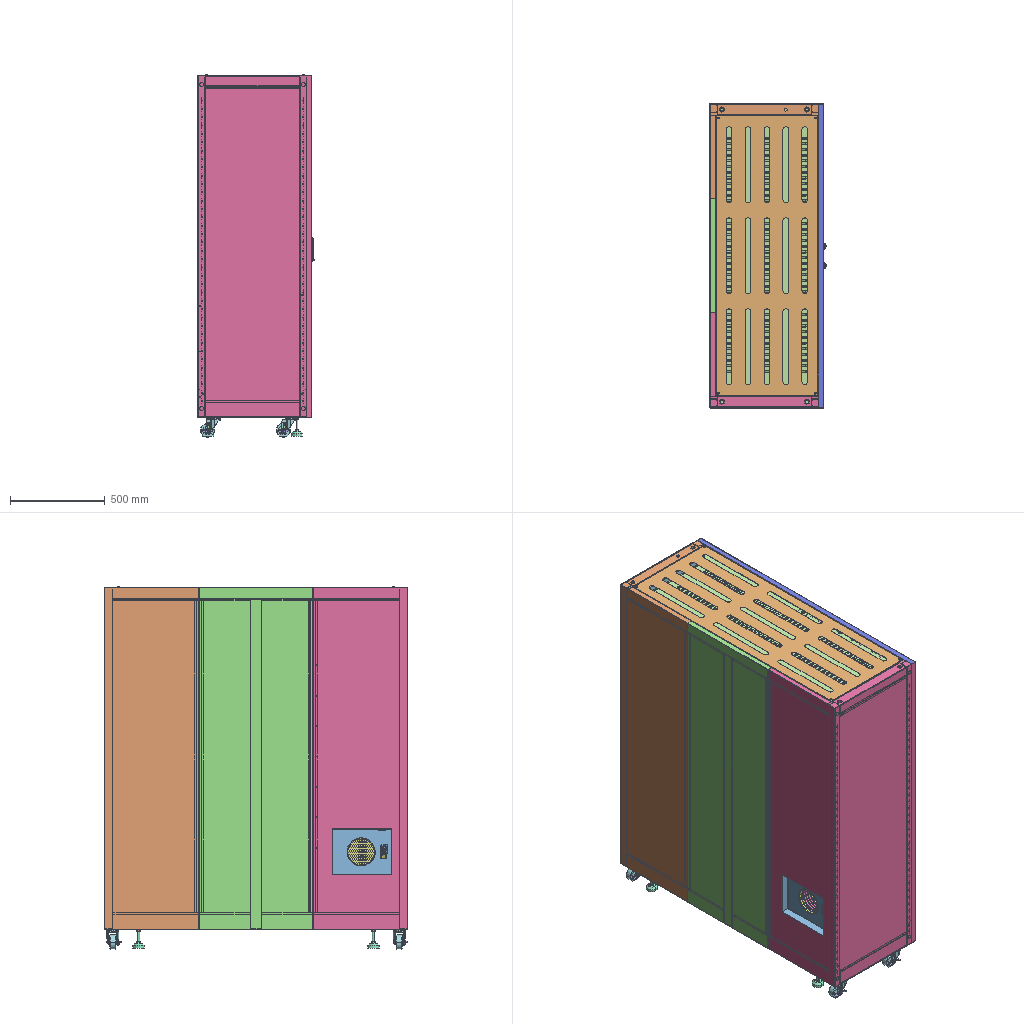Assembly | STEP file | 735 different items | 986 placed | box 612 x 1600 x 1911 mm
Parts list (item | name | quantity | parent item | size | volume), first 254 of 735 items:
1 | - | x1 | in RJWD-DY-0104_000_ASM | 10 x 10 x 37.975 mm | 923.659 mm3
2 | - | x1 | in RJWD-DY-0104_000_ASM | 10 x 10 x 37.975 mm | 923.659 mm3
3 | - | x1 | in RJWD-DY-0104_000_ASM | 10 x 10 x 37.975 mm | 923.659 mm3
4 | - | x1 | in RJWD-DY-0104_000_ASM | 2 x 2 x 1 mm | 3.142 mm3
5 | - | x1 | in RJWD-DY-0104_000_ASM | 2 x 2 x 1 mm | 3.142 mm3
6 | - | x1 | in RJWD-DY-0104_000_ASM | 537 x 1477 x 19.5 mm | 715905 mm3
7 | - | x1 | in RJWD-DY-0104_000_ASM | 10 x 10 x 37.975 mm | 923.659 mm3
8 | - | x1 | in RJWD-DY-0104_000_ASM | 2 x 2 x 1 mm | 3.142 mm3
9 | - | x1 | in RJWD-DY-0104_000_ASM | 2 x 2 x 1 mm | 3.142 mm3
10 | - | x1 | in RJWD-DY-0101_00_ASM | 498 x 92 x 78 mm | 361072 mm3
11 | - | x1 | in RJWD-DY-0101_00_ASM | 12 x 44 x 1659 mm | 107041 mm3
12 | - | x1 | in RJWD-DY-0101_00_ASM | 20 x 20 x 1.5 mm | 532.02 mm3
13 | - | x1 | in RJWD-DY-0101_00_ASM | 32 x 1480 x 131 mm | 236738 mm3
14 | - | x1 | in RJWD-DY-0101_00_ASM | 20 x 20 x 1.5 mm | 532.02 mm3
15 | - | x1 | in RJWD-DY-0101_00_ASM | 40.001 x 1598 x 110 mm | 311237 mm3
16 | - | x1 | in RJWD-DY-0101_00_ASM | 572.5 x 1598 x 16 mm | 960867 mm3
17 | RJWD-DY-0101_0002 | x5 | in RJWD-DY-0101_00_ASM | 10 x 70 x 10 mm | 871.577 mm3
18 | - | x1 | in RJWD-DY-0101_00_ASM | 24 x 27.713 x 13 mm | 3389 mm3
19 | - | x1 | in RJWD-DY-0101_00_ASM | 18 x 20.785 x 10.8 mm | 1989 mm3
20 | SOLID | x4 | in RJWD-DY-0101_300 | 37 x 45 x 1797 mm | 330738 mm3
21 | COMPOUND | x4 | in RJWD-DY-0101_300 | - | -
22 | - | x1 | in RJWD-DY-0101_00_ASM | 18 x 20.785 x 10.8 mm | 1989 mm3
23 | - | x1 | in RJWD-DY-0101_00_ASM | 104 x 1437 x 78 mm | 1081502 mm3
24 | - | x1 | in RJWD-DY-0101_00_ASM | 498 x 55 x 50 mm | 161185 mm3
25 | SOLID | x1 | - | 37 x 60 x 1739 mm | 359493 mm3
26 | COMPOUND | x1 | - | - | -
27 | - | x1 | in RJWD-DY-0101_00_ASM | 18 x 20.785 x 10.8 mm | 1989 mm3
28 | SOLID | x1 | - | 599 x 1598 x 90 mm | 1123369 mm3
29 | COMPOUND | x1 | - | - | -
30 | - | x1 | in RJWD-DY-0101_00_ASM | 600.001 x 500.001 x 1800 mm | 2227675 mm3
31 | - | x1 | in RJWD-DY-0101_00_ASM | 479 x 70 x 30 mm | 90339 mm3
32 | - | x1 | in RJWD-DY-0101_00_ASM | 40 x 600 x 1800 mm | 1173375 mm3
33 | - | x1 | in RJWD-DY-0101_00_ASM | 600.001 x 500.001 x 1800 mm | 2178717 mm3
34 | - | x1 | in RJWD-DY-0101_00_ASM | 479 x 70 x 30 mm | 90339 mm3
35 | - | x1 | in RJWD-DY-0101_00_ASM | 18 x 20.785 x 10.8 mm | 1989 mm3
36 | - | x1 | in RJWD-DY-0101_00_ASM | 498 x 80.2 x 78 mm | 347718 mm3
37 | - | x1 | in RJWD-DY-0101_00_ASM | 12 x 44 x 1659 mm | 107041 mm3
38 | - | x1 | in RJWD-DY-0101_00_ASM | 24 x 27.713 x 13 mm | 3389 mm3
39 | - | x1 | in RJWD-DY-0101_00_ASM | 498 x 55 x 50 mm | 160582 mm3
40 | - | x1 | in RJWD-DY-0101_00_ASM | 24 x 27.713 x 13 mm | 3389 mm3
41 | - | x1 | in RJWD-DY-0101_00_ASM | 37 x 60 x 1739 mm | 359909 mm3
42 | - | x1 | in RJWD-DY-0101_00_ASM | 20 x 20 x 1.5 mm | 532.02 mm3
43 | - | x1 | in RJWD-DY-0101_00_ASM | 20 x 20 x 1.5 mm | 532.02 mm3
44 | - | x1 | in RJWD-DY-0101_00_ASM | 24 x 27.713 x 13 mm | 3389 mm3
45 | - | x1 | in RJWD-DY-0101_00_ASM | 104 x 1437 x 78 mm | 1081502 mm3
46 | RJWD-DY-0101_0003 | x3 | in RJWD-DY-0101_00_ASM | 220 x 15 x 20 mm | 3858 mm3
47 | RJWD-DY-01010001 | x1 | in RJWD-DY-0101_00_ASM | 312.4 x 242.4 x 75 mm | 132718 mm3
48 | - | x1 | in RJWD-DY-0101_00_ASM | 10 x 60 x 10 mm | 771.555 mm3
49 | _GFEEA-D60-M12-L125-DUMMY | x4 | in GFEEA-D60-M12-L125_1_ASM | - | -
50 | _GFEEA-D60-M12-L125-1 | x4 | in GFEEA-D60-M12-L125_1_ASM | 60 x 157 x 60 mm | 76084 mm3
51 | _GFEEA-D60-M12-L125-2 | x4 | in GFEEA-D60-M12-L125_1_ASM | 19 x 10 x 21.939 mm | 2279 mm3
52 | JDC-75-3 | x4 | in JDC-75_ASM | 74.72 x 27.5 x 19.44 mm | 3290 mm3
53 | JDC-75-2 | x4 | in JDC-75_ASM | 25.398 x 59.274 x 36 mm | 3330 mm3
54 | JDC-75-5 | x4 | in JDC-75_ASM | 11.547 x 10 x 3.2 mm | 211.321 mm3
55 | JDC-75-1 | x4 | in JDC-75_ASM | 122 x 106 x 67 mm | 215545 mm3
56 | JDC-75-4 | x4 | in JDC-75_ASM | 6 x 7 x 6 mm | 146.084 mm3
57 | 0001 | x1 | in RJWD-DY-0101_00_ASM | 10 x 10 x 520 mm | 9724 mm3
58 | SOLID | x1 | in 0002 | 48 x 270 x 317 mm | 394936 mm3
59 | COMPOUND | x1 | in 0002 | - | -
60 | RJWD-DY-0101_30002 | x2 | in RJWD-DY-0101_00_ASM | 150 x 10 x 20 mm | 1872 mm3
61 | RJWD-DY-0101_20001 | x2 | in RJWD-DY-0101_00_ASM, RJWD-DY-0115-0001_ASM | 120 x 10 x 20 mm | 1571 mm3
62 | SOLID | x4 | in M1000 | 18.475 x 16 x 9.5 mm | 1567 mm3
63 | SHELL | x4 | in M1000 | - | -
64 | 000 | x1 | in RJWD-DY-0101_00_ASM | 300 x 220 x 20 mm | 1310952 mm3
65 | RJWD-DY-0111_00 | x3 | in RJWD-DY-01_0001_ASM | 24 x 537.5 x 71.5 mm | 60134 mm3
66 | SOLID | x1 | in RJWD-DY-0108_000 | 493 x 75 x 702 mm | 761842 mm3
67 | COMPOUND | x1 | in RJWD-DY-0108_000 | - | -
68 | RJWD-DY-0108_0003 | x4 | in RJWD-DY-0108_000_ASM | 38 x 1 x 20 mm | 730.064 mm3
69 | _2000 | x2 | in RJWD-DY-0108_000_ASM | 426.4 x 3 x 60.8 mm | 11438 mm3
70 | _3000 | x1 | in RJWD-DY-0108_000_ASM | 426.4 x 3 x 60.8 mm | 12335 mm3
71 | _0-1000 | x1 | in RJWD-DY-0108_000_ASM | 278 x 12 x 188 mm | 42731 mm3
72 | M40001 | x12 | in RJWD-DY-0108_000_ASM | 7.9 x 7.9 x 2.97 mm | 98.242 mm3
73 | RJWD-DY-0105--0001 | x1 | in RJWD-DY-0105_-0001_ASM | 728.7 x 458 x 509.2 mm | 1538586 mm3
74 | RJWD-DY-010607_3D0001 | x28 | in RJWD-DY-0105_-0001_ASM, RJWD-DY-0106_-0001_ASM, RJWD-DY-0107_-0001_ASM | 78.111 x 40 x 80.345 mm | 35899 mm3
75 | RJWD-DY-0109_-0001 | x1 | in RJWD-DY-0109_0001_ASM | 722 x 555.2 x 25 mm | 417115 mm3
76 | RJWD-DY-0112_X2_4F20611F56685_1 | x1 | in RJWD-DY-0112_0001_ASM | 1 x 166 x 30 mm | 4869 mm3
77 | RJWD-DY-0112_X2_4F20611F56685_2 | x1 | in RJWD-DY-0112_0001_ASM | 10.8 x 137.602 x 10 mm | 1934 mm3
78 | RJWD-DY-0114_X2_75356C145B89_10 | x1 | in RJWD-DY-0114_0001_ASM | 113.5 x 434 x 340 mm | 170020 mm3
79 | RJWD-DY-0114_X2_75356C145B898_5 | x2 | in RJWD-DY-0114_0001_ASM | 48.998 x 1 x 99.996 mm | 2450 mm3
80 | RJWD-DY-0114_X2_75356C145B898_7 | x1 | in RJWD-DY-0114_0001_ASM | 10 x 10 x 290 mm | 5331 mm3
81 | RJWD-DY-0106--0001 | x1 | in RJWD-DY-0106_-0001_ASM | 728.7 x 458 x 509.2 mm | 1538585 mm3
82 | RJWD-DY-0107--0001 | x1 | in RJWD-DY-0107_-0001_ASM | 728.7 x 458 x 349.2 mm | 1552661 mm3
83 | - | x1 | - | 4 x 509 x 1099 mm | 2237564 mm3
84 | - | x1 | - | 4 x 509.4 x 200.9 mm | 409354 mm3
85 | _X2_751F4E45_X0_LG003_X2_8-1054 | x1 | in _X2_5DE667DC95E88FDE67469501_X0_ASM | 8.003 x 14 x 760 mm | 36967 mm3
86 | _X2_751F4E45_X0_MS731-1_X2_8F_1 | x2 | in _X2_751F4E45_X0_MS731-1_X2_8FDE_ASM | 14.5 x 17.374 x 15.879 mm | 1874 mm3
87 | _X2_751F4E45_X0_MS731-1_X2_8F_3 | x2 | in _X2_751F4E45_X0_MS731-1_X2_8FDE_ASM | 15.1 x 4.709 x 15.173 mm | 73.288 mm3
88 | _X2_751F4E45_X0_MS731-1_X2_8F_4 | x2 | in _X2_751F4E45_X0_MS731-1_X2_8FDE_ASM | 17.2 x 2.5 x 17.2 mm | 530.64 mm3
89 | _X2_751F4E45_X0_MS731-1_X2_8F_5 | x2 | in _X2_751F4E45_X0_MS731-1_X2_8FDE_ASM | 25.8 x 35.5 x 24.1 mm | 3742 mm3
90 | _X2_751F4E45_X0_MS731-1_X2_8F_6 | x2 | in _X2_751F4E45_X0_MS731-1_X2_8FDE_ASM | 30 x 1 x 128 mm | 892.292 mm3
91 | _X2_751F4E45_X0_MS731-1_X2_8F_7 | x2 | in _X2_751F4E45_X0_MS731-1_X2_8FDE_ASM | 44 x 3 x 18 mm | 1686 mm3
92 | _X2_751F4E45_X0_MS731-1_X2_8F_8 | x2 | in _X2_751F4E45_X0_MS731-1_X2_8FDE_ASM | 17.395 x 18 x 83 mm | 8684 mm3
93 | _X2_751F4E45_X0_MS731-1_X2_8F_9 | x2 | in _X2_751F4E45_X0_MS731-1_X2_8FDE_ASM | 29 x 6 x 35 mm | 2353 mm3
94 | _X2_751F4E45_X0_MS731-1_X2_8_10 | x2 | in _X2_751F4E45_X0_MS731-1_X2_8FDE_ASM | 8.5 x 19.466 x 8.5 mm | 271.985 mm3
95 | _X2_751F4E45_X0_MS731-1_X2_8_11 | x2 | in _X2_751F4E45_X0_MS731-1_X2_8FDE_ASM | 22.3 x 4.5 x 4.5 mm | 158.929 mm3
96 | _X2_751F4E45_X0_MS731-1_X2_8_12 | x2 | in _X2_751F4E45_X0_MS731-1_X2_8FDE_ASM | 12 x 12.2 x 12 mm | 416.607 mm3
97 | _X2_751F4E45_X0_MS731-1_X2_8_13 | x2 | in _X2_751F4E45_X0_MS731-1_X2_8FDE_ASM | 31 x 25.045 x 130 mm | 21766 mm3
98 | _X2_751F4E45_X0_MS731-1_X2_8_14 | x2 | in _X2_751F4E45_X0_MS731-1_X2_8FDE_ASM | 8.5 x 19.466 x 8.5 mm | 271.985 mm3
99 | _X2_751F4E45_X0_MS731-1_X2_8_15 | x2 | in _X2_751F4E45_X0_MS731-1_X2_8FDE_ASM | 27 x 14.4 x 37.3 mm | 4925 mm3
100 | _X2_751F4E45_X0_MS731-1_X2_8_16 | x2 | in _X2_751F4E45_X0_MS731-1_X2_8FDE_ASM | 12 x 12.2 x 12 mm | 416.607 mm3
101 | _X2_751F4E45_X0_MS731-1_X2_8_17 | x2 | in _X2_751F4E45_X0_MS731-1_X2_8FDE_ASM | 7 x 2.3 x 7 mm | 15.077 mm3
102 | _X2_751F4E45_X0_MS731-1_X2_8_18 | x2 | in _X2_751F4E45_X0_MS731-1_X2_8FDE_ASM | 12 x 12.2 x 12 mm | 416.607 mm3
103 | _X2_751F4E45_X0_MS731-1_X2_8_19 | x2 | in _X2_751F4E45_X0_MS731-1_X2_8FDE_ASM | 7 x 2.3 x 7 mm | 15.077 mm3
104 | _X2_751F4E45_X0_MS731-1_X2_8_20 | x2 | in _X2_751F4E45_X0_MS731-1_X2_8FDE_ASM | 17 x 13.5 x 26 mm | 1619 mm3
105 | _X2_751F4E45_X0_MS731-1_X2_8_21 | x2 | in _X2_751F4E45_X0_MS731-1_X2_8FDE_ASM | 10 x 1 x 10 mm | 58.905 mm3
106 | _X2_751F4E45_X0_MS731-1_X2_8_22 | x2 | in _X2_751F4E45_X0_MS731-1_X2_8FDE_ASM | 27 x 11.4 x 37.3 mm | 4808 mm3
107 | _X2_751F4E45_X0_MS731-1_X2_8_23 | x2 | in _X2_751F4E45_X0_MS731-1_X2_8FDE_ASM | 16.8 x 3 x 3 mm | 118.356 mm3
108 | _X2_751F4E45_X0_MS731-1_X2_8_24 | x2 | in _X2_751F4E45_X0_MS731-1_X2_8FDE_ASM | 10 x 1 x 10 mm | 58.905 mm3
109 | _X2_751F4E45_X0_MS731-1_X2_8_25 | x2 | in _X2_751F4E45_X0_MS731-1_X2_8FDE_ASM | 22.757 x 2.5 x 22.757 mm | 558.462 mm3
110 | _X2_751F4E45_X0_MS731-1_X2_8_26 | x2 | in _X2_751F4E45_X0_MS731-1_X2_8FDE_ASM | 5.5 x 5 x 5.5 mm | 41.588 mm3
111 | _X2_751F4E45_X0_MS731-1_X2_8_27 | x2 | in _X2_751F4E45_X0_MS731-1_X2_8FDE_ASM | 17.4 x 26.019 x 28.81 mm | 2994 mm3
112 | _X2_751F4E45_X0_MS731-1_X2_8_29 | x2 | in _X2_751F4E45_X0_MS731-1_X2_8FDE_ASM | 5.5 x 5 x 5.5 mm | 41.588 mm3
113 | _X2_751F4E45_X0_RG004-3_X2_5BFC | x4 | in _X2_5DE667DC95E88FDE67469501_X0_ASM, _X2_53F367DC95E88FDE67469501_X0_ASM | 30 x 20 x 36 mm | 14717 mm3
114 | _X2_751F4E45_X0_LG003_X2_8-1051 | x1 | in _X2_5DE667DC95E88FDE67469501_X0_ASM | 14 x 8.003 x 719 mm | 34906 mm3
115 | - | x1 | in RJWD-DY-0102_000_ASM | 18.5 x 511.5 x 98.4 mm | 54675 mm3
116 | - | x1 | in RJWD-DY-0102_000_ASM | 15 x 4 x 4 mm | 187.056 mm3
117 | - | x1 | in RJWD-DY-0102_000_ASM | 18.5 x 511.5 x 34.7 mm | 20752 mm3
118 | - | x1 | in RJWD-DY-0102_000_ASM | 10 x 527.858 x 25 mm | 17063 mm3
119 | RJWD-DY-0102_X2_5DE667DC95E8_11 | x1 | in RJWD-DY-0102_000_ASM | 15 x 4 x 4 mm | 187.056 mm3
120 | RJWD-DY-0102_X2_5DE667DC95E8_12 | x1 | in RJWD-DY-0102_000_ASM | 10 x 501.004 x 192.504 mm | 49501 mm3
121 | RJWD-DY-0102_X2_5DE667DC95E8_14 | x1 | in RJWD-DY-0102_000_ASM | 11.681 x 8 x 8 mm | 225.554 mm3
122 | RJWD-DY-0102_X2_5DE667DC95E8_17 | x1 | in RJWD-DY-0102_000_ASM | 21 x 756.2 x 1704 mm | 844463 mm3
123 | RJWD-DY-0102_X2_5DE667DC95E8_20 | x1 | in RJWD-DY-0102_000_ASM | 15 x 4 x 4 mm | 187.056 mm3
124 | RJWD-DY-0102_X2_5DE667DC95E8_21 | x1 | in RJWD-DY-0102_000_ASM | 11.681 x 8 x 8 mm | 225.554 mm3
125 | RJWD-DY-0102_X2_5DE667DC95E8_22 | x1 | in RJWD-DY-0102_000_ASM | 10 x 501.011 x 1091 mm | 114606 mm3
126 | RJWD-DY-0102_X2_5DE667DC95E8_24 | x1 | in RJWD-DY-0102_000_ASM | 10 x 10 x 18 mm | 607.492 mm3
127 | RJWD-DY-0102_X2_5DE667DC95E8_25 | x1 | in RJWD-DY-0102_000_ASM | 22 x 6 x 6 mm | 613.658 mm3
128 | RJWD-DY-0102_X2_5DE667DC95E8_26 | x1 | in RJWD-DY-0102_000_ASM | 10 x 25 x 219.358 mm | 6666 mm3
129 | RJWD-DY-0102_X2_5DE667DC95E8_27 | x1 | in RJWD-DY-0102_000_ASM | 11.681 x 8 x 8 mm | 225.554 mm3
130 | RJWD-DY-0102_X2_5DE667DC95E8_28 | x1 | in RJWD-DY-0102_000_ASM | 10 x 25 x 1118 mm | 36787 mm3
131 | RJWD-DY-0102_X2_5DE667DC95E8_30 | x1 | in RJWD-DY-0102_000_ASM | 10 x 24 x 62.5 mm | 2502 mm3
132 | RJWD-DY-0102_X2_5DE667DC95E8_33 | x1 | in RJWD-DY-0102_000_ASM | 11.681 x 8 x 8 mm | 225.554 mm3
133 | RJWD-DY-0102_X2_5DE667DC95E8_34 | x1 | in RJWD-DY-0102_000_ASM | 10 x 25 x 1118 mm | 36787 mm3
134 | RJWD-DY-0102_X2_5DE667DC95E8_35 | x1 | in RJWD-DY-0102_000_ASM | 18.5 x 511.5 x 34.7 mm | 20752 mm3
135 | RJWD-DY-0102_X2_5DE667DC95E8_37 | x1 | in RJWD-DY-0102_000_ASM | 5.7 x 17.85 x 93.35 mm | 2651 mm3
136 | RJWD-DY-0102_X2_5DE667DC95E8_38 | x1 | in RJWD-DY-0102_000_ASM | 22 x 6 x 6 mm | 613.658 mm3
137 | RJWD-DY-0102_X2_5DE667DC95E8_39 | x1 | in RJWD-DY-0102_000_ASM | 10 x 545 x 243 mm | 139493 mm3
138 | RJWD-DY-0102_X2_5DE667DC95E8_41 | x1 | in RJWD-DY-0102_000_ASM | 11.681 x 8 x 8 mm | 225.554 mm3
139 | RJWD-DY-0102_X2_5DE667DC95E8_42 | x1 | in RJWD-DY-0102_000_ASM | 10 x 527.858 x 25 mm | 17063 mm3
140 | RJWD-DY-0102_X2_5DE667DC95E8_44 | x1 | in RJWD-DY-0102_000_ASM | 3 x 752 x 1702 mm | 218115 mm3
141 | RJWD-DY-0102_X2_5DE667DC95E8_45 | x1 | in RJWD-DY-0102_000_ASM | 22 x 6 x 6 mm | 613.658 mm3
142 | RJWD-DY-0102_M4X800 | x28 | in RJWD-DY-0102_000_ASM | 11.681 x 8 x 8 mm | 225.554 mm3
143 | RJWD-DY-0102_X2_5DE667DC95E8_48 | x1 | in RJWD-DY-0102_000_ASM | 11.681 x 8 x 8 mm | 225.554 mm3
144 | RJWD-DY-0102_X2_5DE667DC95E8_49 | x1 | in RJWD-DY-0102_000_ASM | 18.5 x 134.2 x 1677 mm | 204085 mm3
145 | RJWD-DY-0102_X2_5DE667DC95E8_50 | x1 | in RJWD-DY-0102_000_ASM | 22 x 6 x 6 mm | 613.658 mm3
146 | RJWD-DY-0102_X2_5DE667DC95E8_53 | x1 | in RJWD-DY-0102_000_ASM | 10 x 25 x 219.358 mm | 6666 mm3
147 | RJWD-DY-0102_X2_5DE667DC95E8_55 | x1 | in RJWD-DY-0102_000_ASM | 11.681 x 8 x 8 mm | 225.554 mm3
148 | RJWD-DY-0102_X2_5DE667DC95E8_56 | x1 | in RJWD-DY-0102_000_ASM | 30.5 x 133.9 x 1677 mm | 217200 mm3
149 | RJWD-DY-0102_X2_5DE667DC95E8_60 | x1 | in RJWD-DY-0102_000_ASM | 11.681 x 8 x 8 mm | 225.554 mm3
150 | RJWD-DY-0102_X2_5DE667DC95E8_61 | x1 | in RJWD-DY-0102_000_ASM | 18.5 x 511.5 x 98.4 mm | 54675 mm3
151 | RJWD-DY-0102_X2_5DE667DC95E8_64 | x1 | in RJWD-DY-0102_000_ASM | 15 x 4 x 4 mm | 187.056 mm3
152 | - | x1 | - | 4 x 509 x 1099 mm | 2237564 mm3
153 | - | x1 | - | 4 x 509.2 x 201.1 mm | 409600 mm3
154 | - | x1 | in RJWD-DY-0103_000_ASM | 11.681 x 8 x 8 mm | 225.551 mm3
155 | - | x1 | in RJWD-DY-0103_000_ASM | 11.681 x 8 x 8 mm | 225.551 mm3
156 | - | x1 | in RJWD-DY-0103_000_ASM | 11.681 x 8 x 8 mm | 225.554 mm3
157 | - | x1 | in RJWD-DY-0103_000_ASM | 11.681 x 8 x 8 mm | 225.551 mm3
158 | - | x1 | in RJWD-DY-0103_000_ASM | 11.681 x 8 x 8 mm | 225.551 mm3
159 | - | x1 | in RJWD-DY-0103_000_ASM | 3 x 754 x 1702 mm | 218295 mm3
160 | - | x1 | in RJWD-DY-0103_000_ASM | 11.681 x 8 x 8 mm | 225.551 mm3
161 | - | x1 | in RJWD-DY-0103_000_ASM | 11.681 x 8 x 8 mm | 225.551 mm3
162 | - | x1 | in RJWD-DY-0103_000_ASM | 11.681 x 8 x 8 mm | 225.551 mm3
163 | RJWD-DY-0103_X2_53F367DC95E8_10 | x1 | in RJWD-DY-0103_000_ASM | 5.7 x 20.85 x 93.35 mm | 2686 mm3
164 | RJWD-DY-0103_X2_53F367DC95E8_11 | x1 | in RJWD-DY-0103_000_ASM | 11.681 x 8 x 8 mm | 225.551 mm3
165 | RJWD-DY-0103_X2_53F367DC95E8_12 | x1 | in RJWD-DY-0103_000_ASM | 10 x 501.011 x 1091 mm | 114606 mm3
166 | RJWD-DY-0103_X2_53F367DC95E8_13 | x1 | in RJWD-DY-0103_000_ASM | 11.681 x 8 x 8 mm | 225.551 mm3
167 | RJWD-DY-0103_X2_53F367DC95E8_14 | x1 | in RJWD-DY-0103_000_ASM | 11.681 x 8 x 8 mm | 225.551 mm3
168 | RJWD-DY-0103_X2_53F367DC95E8_15 | x1 | in RJWD-DY-0103_000_ASM | 11.681 x 8 x 8 mm | 225.551 mm3
169 | RJWD-DY-0103_X2_53F367DC95E8_16 | x1 | in RJWD-DY-0103_000_ASM | 11.681 x 8 x 8 mm | 225.551 mm3
170 | RJWD-DY-0103_X2_53F367DC95E8_17 | x1 | in RJWD-DY-0103_000_ASM | 10 x 527.858 x 25 mm | 17063 mm3
171 | RJWD-DY-0103_X2_53F367DC95E8_18 | x1 | in RJWD-DY-0103_000_ASM | 11.681 x 8 x 8 mm | 225.551 mm3
172 | RJWD-DY-0103_X2_53F367DC95E8_19 | x1 | in RJWD-DY-0103_000_ASM | 11.681 x 8 x 8 mm | 225.551 mm3
173 | RJWD-DY-0103_X2_53F367DC95E8_20 | x1 | in RJWD-DY-0103_000_ASM | 11.681 x 8 x 8 mm | 225.551 mm3
174 | RJWD-DY-0103_X2_53F367DC95E8_21 | x1 | in RJWD-DY-0103_000_ASM | 11.681 x 8 x 8 mm | 225.551 mm3
175 | RJWD-DY-0103_X2_53F367DC95E8_22 | x1 | in RJWD-DY-0103_000_ASM | 11.681 x 8 x 8 mm | 225.551 mm3
176 | RJWD-DY-0103_X2_53F367DC95E8_23 | x1 | in RJWD-DY-0103_000_ASM | 10 x 545 x 243 mm | 139572 mm3
177 | RJWD-DY-0103_X2_53F367DC95E8_24 | x1 | in RJWD-DY-0103_000_ASM | 10 x 24 x 62.5 mm | 2502 mm3
178 | RJWD-DY-0103_X2_53F367DC95E8_25 | x1 | in RJWD-DY-0103_000_ASM | 10 x 10 x 18 mm | 607.492 mm3
179 | RJWD-DY-0103_X2_53F367DC95E8_26 | x1 | in RJWD-DY-0103_000_ASM | 10 x 25 x 1118 mm | 36806 mm3
180 | RJWD-DY-0103_X2_53F367DC95E8_27 | x1 | in RJWD-DY-0103_000_ASM | 10 x 25 x 219.358 mm | 6666 mm3
181 | RJWD-DY-0103_X2_53F367DC95E8_28 | x1 | in RJWD-DY-0103_000_ASM | 11.681 x 8 x 8 mm | 225.551 mm3
182 | RJWD-DY-0103_X2_53F367DC95E8_29 | x1 | in RJWD-DY-0103_000_ASM | 18.5 x 511.5 x 34.7 mm | 20752 mm3
183 | RJWD-DY-0103_X2_53F367DC95E8_30 | x1 | in RJWD-DY-0103_000_ASM | 11.681 x 8 x 8 mm | 225.551 mm3
184 | RJWD-DY-0103_X2_53F367DC95E8_31 | x1 | in RJWD-DY-0103_000_ASM | 11.681 x 8 x 8 mm | 225.554 mm3
185 | RJWD-DY-0103_X2_53F367DC95E8_32 | x1 | in RJWD-DY-0103_000_ASM | 11.681 x 8 x 8 mm | 225.551 mm3
186 | RJWD-DY-0103_X2_53F367DC95E8_33 | x1 | in RJWD-DY-0103_000_ASM | 11.681 x 8 x 8 mm | 225.551 mm3
187 | RJWD-DY-0103_X2_53F367DC95E8_34 | x1 | in RJWD-DY-0103_000_ASM | 30.5 x 133.9 x 1677 mm | 217200 mm3
188 | RJWD-DY-0103_X2_53F367DC95E8_35 | x1 | in RJWD-DY-0103_000_ASM | 11.681 x 8 x 8 mm | 225.551 mm3
189 | RJWD-DY-0103_X2_53F367DC95E8_36 | x1 | in RJWD-DY-0103_000_ASM | 11.681 x 8 x 8 mm | 225.551 mm3
190 | RJWD-DY-0103_X2_53F367DC95E8_37 | x1 | in RJWD-DY-0103_000_ASM | 11.681 x 8 x 8 mm | 225.551 mm3
191 | RJWD-DY-0103_X2_53F367DC95E8_38 | x1 | in RJWD-DY-0103_000_ASM | 11.681 x 8 x 8 mm | 225.551 mm3
192 | RJWD-DY-0103_X2_53F367DC95E8_39 | x1 | in RJWD-DY-0103_000_ASM | 18.5 x 134.2 x 1677 mm | 204085 mm3
193 | RJWD-DY-0103_X2_53F367DC95E8_40 | x1 | in RJWD-DY-0103_000_ASM | 10 x 25 x 1118 mm | 36806 mm3
194 | RJWD-DY-0103_X2_53F367DC95E8_41 | x1 | in RJWD-DY-0103_000_ASM | 11.681 x 8 x 8 mm | 225.554 mm3
195 | RJWD-DY-0103_X2_53F367DC95E8_42 | x1 | in RJWD-DY-0103_000_ASM | 10 x 527.858 x 25 mm | 17063 mm3
196 | RJWD-DY-0103_X2_53F367DC95E8_43 | x1 | in RJWD-DY-0103_000_ASM | 11.681 x 8 x 8 mm | 225.554 mm3
197 | RJWD-DY-0103_X2_53F367DC95E8_44 | x1 | in RJWD-DY-0103_000_ASM | 11.681 x 8 x 8 mm | 225.551 mm3
198 | RJWD-DY-0103_X2_53F367DC95E8_45 | x1 | in RJWD-DY-0103_000_ASM | 18.5 x 511.5 x 34.7 mm | 20752 mm3
199 | RJWD-DY-0103_X2_53F367DC95E8_46 | x1 | in RJWD-DY-0103_000_ASM | 11.681 x 8 x 8 mm | 225.551 mm3
200 | RJWD-DY-0103_X2_53F367DC95E8_47 | x1 | in RJWD-DY-0103_000_ASM | 10 x 25 x 219.358 mm | 6666 mm3
201 | RJWD-DY-0103_X2_53F367DC95E8_48 | x1 | in RJWD-DY-0103_000_ASM | 26.5 x 775.2 x 1704 mm | 873122 mm3
202 | RJWD-DY-0103_X2_53F367DC95E8_49 | x1 | in RJWD-DY-0103_000_ASM | 10 x 501.004 x 192.504 mm | 49501 mm3
203 | RJWD-DY-0103_X2_53F367DC95E8_50 | x1 | in RJWD-DY-0103_000_ASM | 11.681 x 8 x 8 mm | 225.551 mm3
204 | RJWD-DY-0103_X2_53F367DC95E8_51 | x1 | in RJWD-DY-0103_000_ASM | 18.5 x 511.5 x 98.4 mm | 54675 mm3
205 | RJWD-DY-0103_X2_53F367DC95E8_52 | x1 | in RJWD-DY-0103_000_ASM | 11.681 x 8 x 8 mm | 225.551 mm3
206 | RJWD-DY-0103_X2_53F367DC95E8_53 | x1 | in RJWD-DY-0103_000_ASM | 11.681 x 8 x 8 mm | 225.551 mm3
207 | RJWD-DY-0103_X2_53F367DC95E8_54 | x1 | in RJWD-DY-0103_000_ASM | 11.681 x 8 x 8 mm | 225.551 mm3
208 | RJWD-DY-0103_X2_53F367DC95E8_55 | x1 | in RJWD-DY-0103_000_ASM | 11.681 x 8 x 8 mm | 225.551 mm3
209 | RJWD-DY-0103_X2_53F367DC95E8_56 | x1 | in RJWD-DY-0103_000_ASM | 18.5 x 511.5 x 98.4 mm | 54675 mm3
210 | RJWD-DY-0115-0002 | x1 | in RJWD-DY-0115-0001_ASM | 291 x 201 x 191.2 mm | 195011 mm3
211 | RJWD-DY-0113--0001 | x1 | in RJWD-DY-01_0001_ASM | 152 x 132 x 1 mm | 18679 mm3
212 | RJWD-DY-0110_0002 | x1 | in RJWD-DY-0110_0001_ASM | 720 x 548 x 32 mm | 426784 mm3
213 | CHAXIAO6-2_86_1 | x1 | in CHAXIAO6-2_86_ASM | 62.5 x 24 x 10 mm | 2502 mm3
214 | CHAXIAO6-2_86_2 | x1 | in CHAXIAO6-2_86_ASM | 93.35 x 17.85 x 5.7 mm | 2651 mm3
215 | CHAXIAO6-1_78_1 | x1 | in CHAXIAO6-1_78_ASM | 62.5 x 24 x 10 mm | 2502 mm3
216 | CHAXIAO6-1_78_2 | x1 | in CHAXIAO6-1_78_ASM | 93.35 x 20.85 x 5.7 mm | 2686 mm3
217 | SOLID | x9 | in ISO7045-M4X12-4_8 | 15.088 x 8 x 8 mm | 268.486 mm3
218 | SHELL | x9 | in ISO7045-M4X12-4_8 | - | -
219 | DINENISO7092-4 | x13 | in RJWD-DY-01_0001_ASM, 00-RJWD-DY_-10280001_ASM | 0.55 x 8 x 8 mm | 19.659 mm3
220 | DMG10600T070_01WTC_X2_8FEA658_1 | x1 | in DMG10600T070_01WTC_X2_8FEA65875_ASM | 99.7 x 164.6 x 1.775 mm | 25129 mm3
221 | DMG10600T070_01WTC_X2_8FEA658_2 | x1 | in DMG10600T070_01WTC_X2_8FEA65875_ASM | 105.41 x 190.5 x 13.675 mm | 120263 mm3
222 | DMG10600T070_01WTC_X2_8FEA658_3 | x1 | in DMG10600T070_01WTC_X2_8FEA65875_ASM | 105.41 x 190.5 x 7.4 mm | 40629 mm3
223 | DMG10600T070_01WTC_X2_8FEA658_4 | x1 | in DMG10600T070_01WTC_X2_8FEA65875_ASM | 101.5 x 166.2 x 8.5 mm | 2112 mm3
224 | DMG10600T070_01WTC_X2_8FEA658_5 | x1 | in DMG10600T070_01WTC_X2_8FEA65875_ASM | 99.96 x 164.86 x 3.3 mm | 52395 mm3
225 | RJ-HMS7-01_X2_58F34F5394A391D_2 | x1 | in RJ-HMS7-01_X2_58F34F5394A391D17_ASM | 2 x 200 x 140 mm | 19939 mm3
226 | RJ-HMS7-01_X2_58F34F5394A391D_4 | x1 | in RJ-HMS7-01_X2_58F34F5394A391D17_ASM | 1 x 180 x 110 mm | 6715 mm3
227 | RJ-HMS7-01_X2_58F34F5394A391D_1 | x1 | in RJ-HMS7-01_X2_58F34F5394A391D17_ASM | 5.5 x 5.39 x 5.39 mm | 86.619 mm3
228 | RJ-HMS7-01_X2_58F34F5394A391D_3 | x1 | in RJ-HMS7-01_X2_58F34F5394A391D17_ASM | 5.5 x 5.39 x 5.39 mm | 86.619 mm3
229 | RJ-HMS7-01_X2_58F34F5394A391D_5 | x1 | in RJ-HMS7-01_X2_58F34F5394A391D17_ASM | 5.5 x 5.39 x 5.39 mm | 86.619 mm3
230 | RJ-HMS7-01_X2_58F34F5394A391D_6 | x1 | in RJ-HMS7-01_X2_58F34F5394A391D17_ASM | 5.5 x 5.39 x 5.39 mm | 86.619 mm3
231 | ASSEMBLY_GB_T_9074_4_M3X8_2 | x4 | - | 0.8 x 5.4 x 5.4 mm | 12.217 mm3
232 | ASSEMBLY_GB_T_9074_4_M3X8_1 | x4 | - | 10.37 x 5.6 x 5.6 mm | 101.769 mm3
233 | ASSEMBLY_GB_T_9074_4_M3X8_3 | x4 | - | 0.5 x 7 x 7 mm | 14.703 mm3
234 | - | x1 | in RJ-HMS7_0001_ASM | 0.3 x 164.6 x 99.7 mm | 464.94 mm3
235 | 0004 | x1 | in 00-RJWD-DY_-10280001_ASM | 30.6 x 29.06 x 50.3 mm | 18939 mm3
236 | LRS-150-12_X2_5F00517375-151316 | x1 | in LRS-150-12_0001_ASM | 26 x 10.1 x 9.6 mm | 553.854 mm3
237 | LRS-150-12_X2_5F00517375-151317 | x1 | in LRS-150-12_0001_ASM | 18 x 69.7 x 15 mm | 13984 mm3
238 | LRS-150-12_X2_5F00517375-151318 | x1 | in LRS-150-12_0001_ASM | 5 x 0.8 x 15.4 mm | 34.72 mm3
239 | LRS-150-12_X2_5F00517375-151319 | x1 | in LRS-150-12_0001_ASM | 5 x 3 x 3 mm | 26.456 mm3
240 | LRS-150-12_X2_5F00517375-151320 | x1 | in LRS-150-12_0001_ASM | 16.5 x 21.6 x 9 mm | 224.283 mm3
241 | LRS-150-12_X2_5F00517375-151321 | x1 | in LRS-150-12_0001_ASM | 3.75 x 25 x 25.9 mm | 1346 mm3
242 | LRS-150-12_X2_5F00517375-151322 | x1 | in LRS-150-12_0001_ASM | 10.16 x 5.029 x 25.5 mm | 574.438 mm3
243 | LRS-150-12_X2_5F00517375-151323 | x1 | in LRS-150-12_0001_ASM | 6.5 x 6.5 x 5 mm | 70.313 mm3
244 | LRS-150-12_X2_5F00517375-151324 | x1 | in LRS-150-12_0001_ASM | 159 x 97 x 29.5 mm | 32928 mm3
245 | LRS-150-12_X2_5F00517375-151325 | x1 | in LRS-150-12_0001_ASM | 147.5 x 95.25 x 28.5 mm | 5369 mm3
246 | LRS-150-12_X2_5F00517375-151326 | x1 | in LRS-150-12_0001_ASM | 6.5 x 6.5 x 7 mm | 95.446 mm3
247 | LRS-150-12_X2_5F00517375-151327 | x1 | in LRS-150-12_0001_ASM | 5.029 x 10.16 x 25.5 mm | 574.438 mm3
248 | LRS-150-12_X2_5F00517375-151328 | x1 | in LRS-150-12_0001_ASM | 2.65 x 2.65 x 0.4 mm | 2.206 mm3
249 | LRS-150-12_X2_5F00517375-151329 | x1 | in LRS-150-12_0001_ASM | 157 x 93.4 x 0.4 mm | 5710 mm3
250 | LRS-150-12_X2_5F00517375-151330 | x1 | in LRS-150-12_0001_ASM | 5.029 x 10.16 x 25.5 mm | 574.438 mm3
251 | LRS-150-12_X2_5F00517375-151331 | x1 | in LRS-150-12_0001_ASM | 2.65 x 2.65 x 0.4 mm | 2.206 mm3
252 | LRS-150-12_X2_5F00517375-151332 | x1 | in LRS-150-12_0001_ASM | 10.16 x 5.029 x 25.5 mm | 574.438 mm3
253 | LRS-150-12_X2_5F00517375-151333 | x1 | in LRS-150-12_0001_ASM | 16.9 x 32 x 18.5 mm | 618.141 mm3
254 | LRS-150-12_X2_5F00517375-151334 | x1 | in LRS-150-12_0001_ASM | 152 x 94.4 x 1.6 mm | 22494 mm3
Placements (level | parent | child | x y z in mm | rotation matrix by rows), first 186 of 1098 lines:
1 | 00-RJWD-DY_-10280001_ASM | RJWD-DY-01_0001_ASM | 470.0 4439.2 899.144 | 0 1 0 1 0 0 0 0 -1
2 | RJWD-DY-01_0001_ASM | RJWD-DY-0104_000_ASM | -5800.573 800.572 899.144 | 0 1 0 1 0 0 0 0 -1
3 | RJWD-DY-0104_000_ASM | subassembly 2 | 0.0 0.0 0.0 | 1 0 0 0 1 0 0 0 1
3 | RJWD-DY-0104_000_ASM | subassembly 3 | 0.0 0.0 0.0 | 1 0 0 0 1 0 0 0 1
3 | RJWD-DY-0104_000_ASM | subassembly 4 | 0.0 0.0 0.0 | 1 0 0 0 1 0 0 0 1
3 | RJWD-DY-0104_000_ASM | subassembly 5 | 0.0 0.0 0.0 | 1 0 0 0 1 0 0 0 1
3 | RJWD-DY-0104_000_ASM | subassembly 6 | 0.0 0.0 0.0 | 1 0 0 0 1 0 0 0 1
3 | RJWD-DY-0104_000_ASM | subassembly 7 | 0.0 0.0 0.0 | 1 0 0 0 1 0 0 0 1
3 | RJWD-DY-0104_000_ASM | subassembly 8 | 0.0 0.0 0.0 | 1 0 0 0 1 0 0 0 1
3 | RJWD-DY-0104_000_ASM | subassembly 9 | 0.0 0.0 0.0 | 1 0 0 0 1 0 0 0 1
3 | RJWD-DY-0104_000_ASM | subassembly 10 | 0.0 0.0 0.0 | 1 0 0 0 1 0 0 0 1
2 | RJWD-DY-01_0001_ASM | RJWD-DY-0101_00_ASM | -5800.573 800.572 899.144 | 0 1 0 1 0 0 0 0 -1
3 | RJWD-DY-0101_00_ASM | subassembly 11 | 0.0 0.0 0.0 | 1 0 0 0 1 0 0 0 1
3 | RJWD-DY-0101_00_ASM | subassembly 12 | 0.0 0.0 0.0 | 1 0 0 0 1 0 0 0 1
3 | RJWD-DY-0101_00_ASM | subassembly 13 | 0.0 0.0 0.0 | 1 0 0 0 1 0 0 0 1
3 | RJWD-DY-0101_00_ASM | subassembly 14 | 0.0 0.0 0.0 | 1 0 0 0 1 0 0 0 1
3 | RJWD-DY-0101_00_ASM | subassembly 15 | 0.0 0.0 0.0 | 1 0 0 0 1 0 0 0 1
3 | RJWD-DY-0101_00_ASM | subassembly 16 | 0.0 0.0 0.0 | 1 0 0 0 1 0 0 0 1
3 | RJWD-DY-0101_00_ASM | subassembly 17 | 0.0 0.0 0.0 | 1 0 0 0 1 0 0 0 1
3 | RJWD-DY-0101_00_ASM | RJWD-DY-0101_0002 | 0.0 -170.0 0.0 | 1 0 0 0 1 0 0 0 1
3 | RJWD-DY-0101_00_ASM | RJWD-DY-0101_0002 | 0.0 -320.0 0.0 | 1 0 0 0 1 0 0 0 1
3 | RJWD-DY-0101_00_ASM | RJWD-DY-0101_0002 | 0.0 -470.0 0.0 | 1 0 0 0 1 0 0 0 1
3 | RJWD-DY-0101_00_ASM | RJWD-DY-0101_0002 | 0.0 -620.0 0.0 | 1 0 0 0 1 0 0 0 1
3 | RJWD-DY-0101_00_ASM | RJWD-DY-0101_0002 | 0.0 -770.0 0.0 | 1 0 0 0 1 0 0 0 1
3 | RJWD-DY-0101_00_ASM | subassembly 18 | 0.0 0.0 0.0 | 1 0 0 0 1 0 0 0 1
3 | RJWD-DY-0101_00_ASM | subassembly 19 | 0.0 0.0 0.0 | 1 0 0 0 1 0 0 0 1
3 | RJWD-DY-0101_00_ASM | RJWD-DY-0101_300 | 0.0 0.0 0.0 | 1 0 0 0 1 0 0 0 1
4 | RJWD-DY-0101_300 | SOLID | 0.0 0.0 0.0 | 1 0 0 0 1 0 0 0 1
4 | RJWD-DY-0101_300 | COMPOUND | 0.0 0.0 0.0 | 1 0 0 0 1 0 0 0 1
3 | RJWD-DY-0101_00_ASM | RJWD-DY-0101_300 | -1626.145 11556.145 0.0 | -1 0 0 0 -1 0 0 0 1
4 | RJWD-DY-0101_300 | SOLID | 0.0 0.0 0.0 | 1 0 0 0 1 0 0 0 1
4 | RJWD-DY-0101_300 | COMPOUND | 0.0 0.0 0.0 | 1 0 0 0 1 0 0 0 1
3 | RJWD-DY-0101_00_ASM | RJWD-DY-0101_300 | 0.0 -1553.0 0.0 | 1 0 0 0 1 0 0 0 1
4 | RJWD-DY-0101_300 | SOLID | 0.0 0.0 0.0 | 1 0 0 0 1 0 0 0 1
4 | RJWD-DY-0101_300 | COMPOUND | 0.0 0.0 0.0 | 1 0 0 0 1 0 0 0 1
3 | RJWD-DY-0101_00_ASM | RJWD-DY-0101_300 | -1626.145 10003.145 0.0 | -1 0 0 0 -1 0 0 0 1
4 | RJWD-DY-0101_300 | SOLID | 0.0 0.0 0.0 | 1 0 0 0 1 0 0 0 1
4 | RJWD-DY-0101_300 | COMPOUND | 0.0 0.0 0.0 | 1 0 0 0 1 0 0 0 1
3 | RJWD-DY-0101_00_ASM | subassembly 20 | 0.0 0.0 0.0 | 1 0 0 0 1 0 0 0 1
3 | RJWD-DY-0101_00_ASM | subassembly 21 | 0.0 0.0 0.0 | 1 0 0 0 1 0 0 0 1
3 | RJWD-DY-0101_00_ASM | subassembly 22 | 0.0 0.0 0.0 | 1 0 0 0 1 0 0 0 1
3 | RJWD-DY-0101_00_ASM | subassembly 23 | 0.0 0.0 0.0 | 1 0 0 0 1 0 0 0 1
4 | subassembly 23 | SOLID | 0.0 0.0 0.0 | 1 0 0 0 1 0 0 0 1
4 | subassembly 23 | COMPOUND | 0.0 0.0 0.0 | 1 0 0 0 1 0 0 0 1
3 | RJWD-DY-0101_00_ASM | subassembly 24 | 0.0 0.0 0.0 | 1 0 0 0 1 0 0 0 1
3 | RJWD-DY-0101_00_ASM | subassembly 25 | 0.0 0.0 0.0 | 1 0 0 0 1 0 0 0 1
4 | subassembly 25 | SOLID | 0.0 0.0 0.0 | 1 0 0 0 1 0 0 0 1
4 | subassembly 25 | COMPOUND | 0.0 0.0 0.0 | 1 0 0 0 1 0 0 0 1
3 | RJWD-DY-0101_00_ASM | subassembly 26 | 0.0 0.0 0.0 | 1 0 0 0 1 0 0 0 1
3 | RJWD-DY-0101_00_ASM | subassembly 27 | 0.0 0.0 0.0 | 1 0 0 0 1 0 0 0 1
3 | RJWD-DY-0101_00_ASM | subassembly 28 | 0.0 0.0 0.0 | 1 0 0 0 1 0 0 0 1
3 | RJWD-DY-0101_00_ASM | subassembly 29 | 0.0 0.0 0.0 | 1 0 0 0 1 0 0 0 1
3 | RJWD-DY-0101_00_ASM | subassembly 30 | 0.0 0.0 0.0 | 1 0 0 0 1 0 0 0 1
3 | RJWD-DY-0101_00_ASM | subassembly 31 | 0.0 0.0 0.0 | 1 0 0 0 1 0 0 0 1
3 | RJWD-DY-0101_00_ASM | subassembly 32 | 0.0 0.0 0.0 | 1 0 0 0 1 0 0 0 1
3 | RJWD-DY-0101_00_ASM | subassembly 33 | 0.0 0.0 0.0 | 1 0 0 0 1 0 0 0 1
3 | RJWD-DY-0101_00_ASM | subassembly 34 | 0.0 0.0 0.0 | 1 0 0 0 1 0 0 0 1
3 | RJWD-DY-0101_00_ASM | subassembly 35 | 0.0 0.0 0.0 | 1 0 0 0 1 0 0 0 1
3 | RJWD-DY-0101_00_ASM | subassembly 36 | 0.0 0.0 0.0 | 1 0 0 0 1 0 0 0 1
3 | RJWD-DY-0101_00_ASM | subassembly 37 | 0.0 0.0 0.0 | 1 0 0 0 1 0 0 0 1
3 | RJWD-DY-0101_00_ASM | subassembly 38 | 0.0 0.0 0.0 | 1 0 0 0 1 0 0 0 1
3 | RJWD-DY-0101_00_ASM | subassembly 39 | 0.0 0.0 0.0 | 1 0 0 0 1 0 0 0 1
3 | RJWD-DY-0101_00_ASM | subassembly 40 | 0.0 0.0 0.0 | 1 0 0 0 1 0 0 0 1
3 | RJWD-DY-0101_00_ASM | subassembly 41 | 0.0 0.0 0.0 | 1 0 0 0 1 0 0 0 1
3 | RJWD-DY-0101_00_ASM | RJWD-DY-0101_0003 | -6003.145 3711.0 0.0 | 0 1 0 -1 0 0 0 0 1
3 | RJWD-DY-0101_00_ASM | RJWD-DY-01010001 | -1054.572 4447.573 406.644 | 0 0 -1 -1 0 0 0 1 0
3 | RJWD-DY-0101_00_ASM | subassembly 42 | 0.0 -883.459 253.2 | 1 0 0 0 1 0 0 0 1
3 | RJWD-DY-0101_00_ASM | RJWD-DY-0101_0003 | -146.0 -1114.0 0.0 | 1 0 0 0 1 0 0 0 1
3 | RJWD-DY-0101_00_ASM | RJWD-DY-0101_0003 | 4661.0 5382.145 0.0 | 0 -1 0 1 0 0 0 0 1
3 | RJWD-DY-0101_00_ASM | GFEEA-D60-M12-L125_ASM | -579.072 4382.972 -100.356 | -1 0 0 0 0 1 0 1 0
4 | GFEEA-D60-M12-L125_ASM | GFEEA-D60-M12-L125_1_ASM | 0.0 0.0 0.0 | 1 0 0 0 1 0 0 0 1
5 | GFEEA-D60-M12-L125_1_ASM | _GFEEA-D60-M12-L125-DUMMY | 0.0 0.0 0.0 | 1 0 0 0 1 0 0 0 1
5 | GFEEA-D60-M12-L125_1_ASM | _GFEEA-D60-M12-L125-1 | 0.0 0.0 0.0 | 1 0 0 0 1 0 0 0 1
5 | GFEEA-D60-M12-L125_1_ASM | _GFEEA-D60-M12-L125-2 | 0.0 99.5 0.0 | 1 0 0 0 -1 0 0 0 -1
3 | RJWD-DY-0101_00_ASM | GFEEA-D60-M12-L125_ASM | -1047.072 4382.972 -100.356 | -1 0 0 0 0 1 0 1 0
4 | GFEEA-D60-M12-L125_ASM | GFEEA-D60-M12-L125_1_ASM | 0.0 0.0 0.0 | 1 0 0 0 1 0 0 0 1
5 | GFEEA-D60-M12-L125_1_ASM | _GFEEA-D60-M12-L125-DUMMY | 0.0 0.0 0.0 | 1 0 0 0 1 0 0 0 1
5 | GFEEA-D60-M12-L125_1_ASM | _GFEEA-D60-M12-L125-1 | 0.0 0.0 0.0 | 1 0 0 0 1 0 0 0 1
5 | GFEEA-D60-M12-L125_1_ASM | _GFEEA-D60-M12-L125-2 | 0.0 99.5 0.0 | 1 0 0 0 -1 0 0 0 -1
3 | RJWD-DY-0101_00_ASM | GFEEA-D60-M12-L125_ASM | -579.072 5620.172 -100.356 | -1 0 0 0 0 1 0 1 0
4 | GFEEA-D60-M12-L125_ASM | GFEEA-D60-M12-L125_1_ASM | 0.0 0.0 0.0 | 1 0 0 0 1 0 0 0 1
5 | GFEEA-D60-M12-L125_1_ASM | _GFEEA-D60-M12-L125-DUMMY | 0.0 0.0 0.0 | 1 0 0 0 1 0 0 0 1
5 | GFEEA-D60-M12-L125_1_ASM | _GFEEA-D60-M12-L125-1 | 0.0 0.0 0.0 | 1 0 0 0 1 0 0 0 1
5 | GFEEA-D60-M12-L125_1_ASM | _GFEEA-D60-M12-L125-2 | 0.0 99.5 0.0 | 1 0 0 0 -1 0 0 0 -1
3 | RJWD-DY-0101_00_ASM | GFEEA-D60-M12-L125_ASM | -1047.072 5620.172 -100.356 | -1 0 0 0 0 1 0 1 0
4 | GFEEA-D60-M12-L125_ASM | GFEEA-D60-M12-L125_1_ASM | 0.0 0.0 0.0 | 1 0 0 0 1 0 0 0 1
5 | GFEEA-D60-M12-L125_1_ASM | _GFEEA-D60-M12-L125-DUMMY | 0.0 0.0 0.0 | 1 0 0 0 1 0 0 0 1
5 | GFEEA-D60-M12-L125_1_ASM | _GFEEA-D60-M12-L125-1 | 0.0 0.0 0.0 | 1 0 0 0 1 0 0 0 1
5 | GFEEA-D60-M12-L125_1_ASM | _GFEEA-D60-M12-L125-2 | 0.0 99.5 0.0 | 1 0 0 0 -1 0 0 0 -1
3 | RJWD-DY-0101_00_ASM | subassembly 43 | -626.142 4374.068 -105.027 | 1 0 0 0 0 -1 0 1 0
4 | subassembly 43 | JDC-75_ASM | 0.0 0.0 0.0 | 1 0 0 0 1 0 0 0 1
5 | JDC-75_ASM | JDC-75-3 | -23.375 37.783 154.746 | 0.9995 -0.0322 0 0.0322 0.9995 0 0 0 1
5 | JDC-75_ASM | JDC-75-2 | -23.93 42.445 152.246 | 1 0 0 0 1 0 0 0 1
5 | JDC-75_ASM | JDC-75-5 | -24.43 35.171 157.596 | -0.859 -0.512 0 -0.512 0.859 0 0 0 -1
5 | JDC-75_ASM | JDC-75-1 | -24.43 35.171 126.996 | 1 0 0 0 1 0 0 0 1
5 | JDC-75_ASM | JDC-75-4 | -26.625 22.171 149.996 | 0.3857 0 -0.9226 -0.9226 0 -0.3857 0 1 0
3 | RJWD-DY-0101_00_ASM | subassembly 43 | -1025.142 4374.068 -105.027 | 1 0 0 0 0 -1 0 1 0
4 | subassembly 43 | JDC-75_ASM | 0.0 0.0 0.0 | 1 0 0 0 1 0 0 0 1
5 | JDC-75_ASM | JDC-75-3 | -23.375 37.783 154.746 | 0.9995 -0.0322 0 0.0322 0.9995 0 0 0 1
5 | JDC-75_ASM | JDC-75-2 | -23.93 42.445 152.246 | 1 0 0 0 1 0 0 0 1
5 | JDC-75_ASM | JDC-75-5 | -24.43 35.171 157.596 | -0.859 -0.512 0 -0.512 0.859 0 0 0 -1
5 | JDC-75_ASM | JDC-75-1 | -24.43 35.171 126.996 | 1 0 0 0 1 0 0 0 1
5 | JDC-75_ASM | JDC-75-4 | -26.625 22.171 149.996 | 0.3857 0 -0.9226 -0.9226 0 -0.3857 0 1 0
3 | RJWD-DY-0101_00_ASM | subassembly 43 | -626.142 5883.068 -105.027 | 1 0 0 0 0 -1 0 1 0
4 | subassembly 43 | JDC-75_ASM | 0.0 0.0 0.0 | 1 0 0 0 1 0 0 0 1
5 | JDC-75_ASM | JDC-75-3 | -23.375 37.783 154.746 | 0.9995 -0.0322 0 0.0322 0.9995 0 0 0 1
5 | JDC-75_ASM | JDC-75-2 | -23.93 42.445 152.246 | 1 0 0 0 1 0 0 0 1
5 | JDC-75_ASM | JDC-75-5 | -24.43 35.171 157.596 | -0.859 -0.512 0 -0.512 0.859 0 0 0 -1
5 | JDC-75_ASM | JDC-75-1 | -24.43 35.171 126.996 | 1 0 0 0 1 0 0 0 1
5 | JDC-75_ASM | JDC-75-4 | -26.625 22.171 149.996 | 0.3857 0 -0.9226 -0.9226 0 -0.3857 0 1 0
3 | RJWD-DY-0101_00_ASM | subassembly 43 | -1025.142 5883.068 -105.027 | 1 0 0 0 0 -1 0 1 0
4 | subassembly 43 | JDC-75_ASM | 0.0 0.0 0.0 | 1 0 0 0 1 0 0 0 1
5 | JDC-75_ASM | JDC-75-3 | -23.375 37.783 154.746 | 0.9995 -0.0322 0 0.0322 0.9995 0 0 0 1
5 | JDC-75_ASM | JDC-75-2 | -23.93 42.445 152.246 | 1 0 0 0 1 0 0 0 1
5 | JDC-75_ASM | JDC-75-5 | -24.43 35.171 157.596 | -0.859 -0.512 0 -0.512 0.859 0 0 0 -1
5 | JDC-75_ASM | JDC-75-1 | -24.43 35.171 126.996 | 1 0 0 0 1 0 0 0 1
5 | JDC-75_ASM | JDC-75-4 | -26.625 22.171 149.996 | 0.3857 0 -0.9226 -0.9226 0 -0.3857 0 1 0
3 | RJWD-DY-0101_00_ASM | 0001 | -813.072 4247.573 637.644 | 0 0 -1 -1 0 0 0 1 0
3 | RJWD-DY-0101_00_ASM | 0002 | -824.572 4447.573 126.644 | 0 0 -1 0 1 0 1 0 0
4 | 0002 | SOLID | 0.0 0.0 0.0 | 1 0 0 0 1 0 0 0 1
4 | 0002 | COMPOUND | 0.0 0.0 0.0 | 1 0 0 0 1 0 0 0 1
3 | RJWD-DY-0101_00_ASM | RJWD-DY-0101_30002 | 4824.0 5832.145 -0.0 | 0 -1 0 1 0 0 0 0 1
3 | RJWD-DY-0101_00_ASM | RJWD-DY-0101_30002 | 4824.0 5632.145 -0.0 | 0 -1 0 1 0 0 0 0 1
3 | RJWD-DY-0101_00_ASM | RJWD-DY-0101_20001 | 255.0 -470.0 0.0 | 1 0 0 0 1 0 0 0 1
3 | RJWD-DY-0101_00_ASM | M1000 | -726.31 4507.573 114.144 | 1 0 0 0 1 0 0 0 1
4 | M1000 | SOLID | 0.0 0.0 0.0 | 1 0 0 0 1 0 0 0 1
4 | M1000 | SHELL | 0.0 0.0 0.0 | 1 0 0 0 1 0 0 0 1
3 | RJWD-DY-0101_00_ASM | M1000 | -941.31 4507.573 114.144 | 1 0 0 0 1 0 0 0 1
4 | M1000 | SOLID | 0.0 0.0 0.0 | 1 0 0 0 1 0 0 0 1
4 | M1000 | SHELL | 0.0 0.0 0.0 | 1 0 0 0 1 0 0 0 1
3 | RJWD-DY-0101_00_ASM | M1000 | -726.31 4387.573 114.144 | 1 0 0 0 1 0 0 0 1
4 | M1000 | SOLID | 0.0 0.0 0.0 | 1 0 0 0 1 0 0 0 1
4 | M1000 | SHELL | 0.0 0.0 0.0 | 1 0 0 0 1 0 0 0 1
3 | RJWD-DY-0101_00_ASM | M1000 | -941.31 4387.573 114.144 | 1 0 0 0 1 0 0 0 1
4 | M1000 | SOLID | 0.0 0.0 0.0 | 1 0 0 0 1 0 0 0 1
4 | M1000 | SHELL | 0.0 0.0 0.0 | 1 0 0 0 1 0 0 0 1
3 | RJWD-DY-0101_00_ASM | 000 | -824.572 4447.573 146.644 | 1 0 0 0 -1 0 0 0 -1
2 | RJWD-DY-01_0001_ASM | RJWD-DY-0111_00 | -1598.795 -1484.998 -193.177 | -1 0 0 0 1 0 0 0 -1
2 | RJWD-DY-01_0001_ASM | RJWD-DY-0111_00 | -1598.795 -1484.968 -809.177 | -1 0 0 0 1 0 0 0 -1
2 | RJWD-DY-01_0001_ASM | RJWD-DY-0108_000_ASM | 3741.8 445.0 895.044 | 0 -1 0 -1 0 0 0 0 -1
3 | RJWD-DY-0108_000_ASM | RJWD-DY-0108_000 | 0.0 0.0 0.0 | 1 0 0 0 1 0 0 0 1
4 | RJWD-DY-0108_000 | SOLID | 0.0 0.0 0.0 | 1 0 0 0 1 0 0 0 1
4 | RJWD-DY-0108_000 | COMPOUND | 0.0 0.0 0.0 | 1 0 0 0 1 0 0 0 1
3 | RJWD-DY-0108_000_ASM | RJWD-DY-0108_0003 | -2.0 0.0 -124.1 | 1 0 0 0 1 0 0 0 1
3 | RJWD-DY-0108_000_ASM | RJWD-DY-0108_0003 | -2.0 0.0 400.9 | 1 0 0 0 1 0 0 0 1
3 | RJWD-DY-0108_000_ASM | RJWD-DY-0108_0003 | 917.0 9142.6 -124.1 | -1 0 0 0 -1 0 0 0 1
3 | RJWD-DY-0108_000_ASM | RJWD-DY-0108_0003 | 917.0 9142.6 400.9 | -1 0 0 0 -1 0 0 0 1
3 | RJWD-DY-0108_000_ASM | _2000 | 0.0 0.0 0.0 | 1 0 0 0 1 0 0 0 1
3 | RJWD-DY-0108_000_ASM | _2000 | -0.0039 -59.0 43.963 | 1 0 0 0 1 0 0 0 1
3 | RJWD-DY-0108_000_ASM | _3000 | 916.032 9081.6 -571.998 | -1 0 0 0 -1 0 0 0 1
3 | RJWD-DY-0108_000_ASM | _0-1000 | -2.5 1116.0 -20.5 | 1 0 0 0 1 0 0 0 1
3 | RJWD-DY-0108_000_ASM | M40001 | -1918.984 2329.15 -3842.444 | -1 0 0 0 0 1 0 1 0
3 | RJWD-DY-0108_000_ASM | M40001 | -2038.984 2329.15 -3842.444 | -1 0 0 0 0 1 0 1 0
3 | RJWD-DY-0108_000_ASM | M40001 | -2158.984 2329.15 -3842.444 | -1 0 0 0 0 1 0 1 0
3 | RJWD-DY-0108_000_ASM | M40001 | -2278.984 2329.15 -3842.444 | -1 0 0 0 0 1 0 1 0
3 | RJWD-DY-0108_000_ASM | M40001 | -1918.984 2329.15 -4458.444 | -1 0 0 0 0 1 0 1 0
3 | RJWD-DY-0108_000_ASM | M40001 | -2038.984 2329.15 -4458.444 | -1 0 0 0 0 1 0 1 0
3 | RJWD-DY-0108_000_ASM | M40001 | -2158.984 2329.15 -4458.444 | -1 0 0 0 0 1 0 1 0
3 | RJWD-DY-0108_000_ASM | M40001 | -2278.984 2329.15 -4458.444 | -1 0 0 0 0 1 0 1 0
3 | RJWD-DY-0108_000_ASM | M40001 | 3194.016 6752.45 -3886.446 | 1 0 0 0 0 -1 0 1 0
3 | RJWD-DY-0108_000_ASM | M40001 | 3074.016 6752.45 -3886.446 | 1 0 0 0 0 -1 0 1 0
3 | RJWD-DY-0108_000_ASM | M40001 | 2954.016 6752.45 -3886.446 | 1 0 0 0 0 -1 0 1 0
3 | RJWD-DY-0108_000_ASM | M40001 | 2834.016 6752.45 -3886.446 | 1 0 0 0 0 -1 0 1 0
2 | RJWD-DY-01_0001_ASM | RJWD-DY-0111_00 | 0.7953 1459.928 -765.177 | 1 0 0 0 -1 0 0 0 -1
2 | RJWD-DY-01_0001_ASM | RJWD-DY-0105_-0001_ASM | -1190.75 -12.516 223.75 | 1 0 0 0 -1 0 0 0 -1
3 | RJWD-DY-0105_-0001_ASM | RJWD-DY-0105--0001 | 0.0 0.0 0.0 | 1 0 0 0 1 0 0 0 1
3 | RJWD-DY-0105_-0001_ASM | RJWD-DY-010607_3D0001 | -2658.45 608 32.594 | 0 1 0 -1 0 0 0 0 1
3 | RJWD-DY-0105_-0001_ASM | RJWD-DY-010607_3D0001 | -2818.45 608 32.594 | 0 1 0 -1 0 0 0 0 1
3 | RJWD-DY-0105_-0001_ASM | RJWD-DY-010607_3D0001 | -2978.45 608 32.594 | 0 1 0 -1 0 0 0 0 1
3 | RJWD-DY-0105_-0001_ASM | RJWD-DY-010607_3D0001 | -3138.45 608 32.594 | 0 1 0 -1 0 0 0 0 1
3 | RJWD-DY-0105_-0001_ASM | RJWD-DY-010607_3D0001 | -2738.45 418.2 -17.406 | 0 1 0 -1 0 0 0 0 1
3 | RJWD-DY-0105_-0001_ASM | RJWD-DY-010607_3D0001 | -2898.45 418.2 -17.406 | 0 1 0 -1 0 0 0 0 1
3 | RJWD-DY-0105_-0001_ASM | RJWD-DY-010607_3D0001 | -3058.45 418.2 -17.406 | 0 1 0 -1 0 0 0 0 1
3 | RJWD-DY-0105_-0001_ASM | RJWD-DY-010607_3D0001 | -3218.45 418.2 -17.406 | 0 1 0 -1 0 0 0 0 1
2 | RJWD-DY-01_0001_ASM | RJWD-DY-0109_0001_ASM | -1191.0 255.5 543.5 | 1 0 0 0 0 1 0 -1 0
3 | RJWD-DY-0109_0001_ASM | RJWD-DY-0109_-0001 | 0.0 0.0 0.0 | 1 0 0 0 1 0 0 0 1
2 | RJWD-DY-01_0001_ASM | RJWD-DY-0112_0001_ASM | -125.0 -4695.6 602.544 | -1 0 0 0 1 0 0 0 -1
3 | RJWD-DY-0112_0001_ASM | RJWD-DY-0112_X2_4F20611F56685_1 | 0.0 0.0 0.0 | 1 0 0 0 1 0 0 0 1
3 | RJWD-DY-0112_0001_ASM | RJWD-DY-0112_X2_4F20611F56685_2 | 0.0 10.002 0.0 | 1 0 0 0 1 0 0 0 1
2 | RJWD-DY-01_0001_ASM | RJWD-DY-0114_0001_ASM | -6213.2 -466.291 929.144 | 0 1 0 1 0 0 0 0 -1
3 | RJWD-DY-0114_0001_ASM | RJWD-DY-0114_X2_75356C145B89_10 | 0.0 0.0 0.0 | 1 0 0 0 1 0 0 0 1
3 | RJWD-DY-0114_0001_ASM | RJWD-DY-0114_X2_75356C145B898_5 | 0.002 0.5 -10.0 | 1 0 0 0 1 0 0 0 1
3 | RJWD-DY-0114_0001_ASM | RJWD-DY-0114_X2_75356C145B898_5 | 0.002 -149.5 -10.0 | 1 0 0 0 1 0 0 0 1
3 | RJWD-DY-0114_0001_ASM | RJWD-DY-0114_X2_75356C145B898_7 | 0.0 0.0 0.0 | 1 0 0 0 1 0 0 0 1
2 | RJWD-DY-01_0001_ASM | RJWD-DY-0106_-0001_ASM | -407.25 -12.516 179.737 | -1 0 0 0 1 0 0 0 -1
3 | RJWD-DY-0106_-0001_ASM | RJWD-DY-0106--0001 | 0.0 0.0 0.0 | 1 0 0 0 1 0 0 0 1